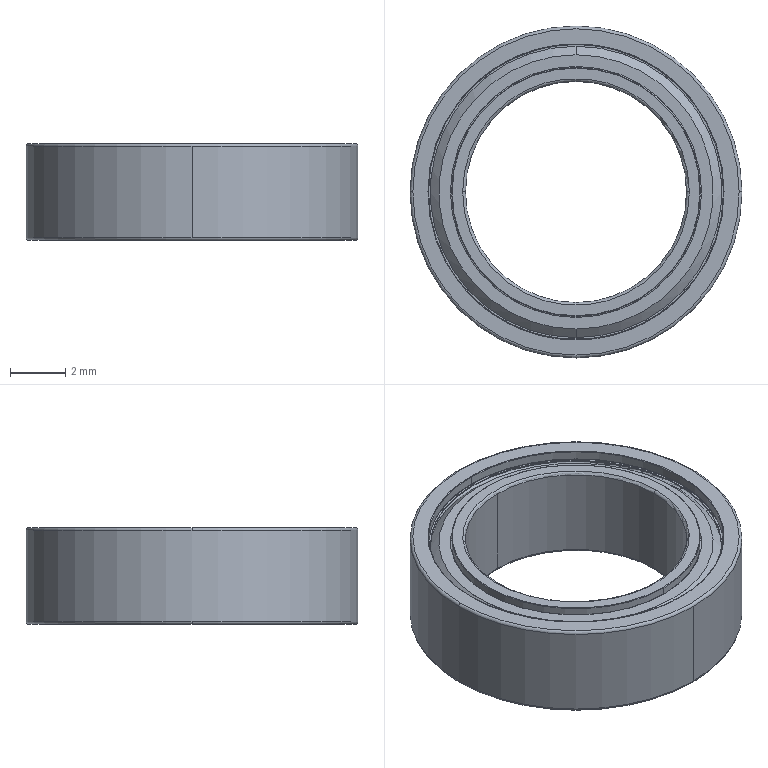Part | SolidWorks | features BaseBody 4 | 4 solids | 339 faces | box 12 x 12 x 3.5 mm | volume 150.581 mm3 | torus 134 | sphere 108 | plane 49 | cylinder 36 | cone 12 | commonest cylinder face diameters 10.667 x8 9 x4 9.081 x4 9.167 x4 9.333 x4 10.538 x4